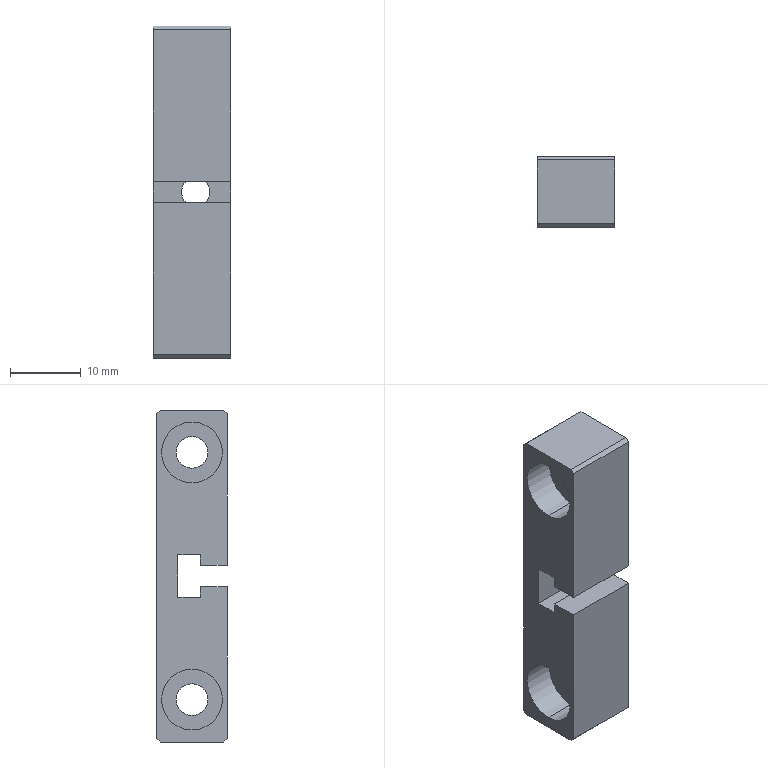Part | NX | features BREP 1 | 1 solid | 30 faces | box 11 x 10 x 47 mm | volume 4061 mm3 | plane 20 | cylinder 10 | commonest cylinder face diameters 4.5 x4 8.6 x4 4 x2
STEP:
#1=CARTESIAN_POINT('',(-1.,0.,-21.8));
#2=VERTEX_POINT('',#1);
#3=CARTESIAN_POINT('',(-1.,0.,-13.2));
#4=VERTEX_POINT('',#3);
#5=CARTESIAN_POINT('',(-1.,0.,-17.5));
#6=DIRECTION('',(-1.,0.,0.));
#7=DIRECTION('',(0.,0.,1.));
#8=AXIS2_PLACEMENT_3D('',#5,#6,#7);
#9=CIRCLE('',#8,4.3);
#10=EDGE_CURVE('',#2,#4,#9,.T.);
#11=ORIENTED_EDGE('',*,*,#10,.F.);
#12=CARTESIAN_POINT('',(-5.5,0.,-21.8));
#13=VERTEX_POINT('',#12);
#14=CARTESIAN_POINT('',(-5.5,0.,-21.8));
#15=DIRECTION('',(-1.,0.,0.));
#16=VECTOR('',#15,1000.);
#17=LINE('',#14,#16);
#18=EDGE_CURVE('',#13,#2,#17,.F.);
#19=ORIENTED_EDGE('',*,*,#18,.F.);
#20=CARTESIAN_POINT('',(-5.5,0.,-13.2));
#21=VERTEX_POINT('',#20);
#22=CARTESIAN_POINT('',(-5.5,0.,-17.5));
#23=DIRECTION('',(-1.,0.,0.));
#24=DIRECTION('',(0.,0.,1.));
#25=AXIS2_PLACEMENT_3D('',#22,#23,#24);
#26=CIRCLE('',#25,4.3);
#27=EDGE_CURVE('',#13,#21,#26,.T.);
#28=ORIENTED_EDGE('',*,*,#27,.T.);
#29=CARTESIAN_POINT('',(-5.5,0.,-13.2));
#30=DIRECTION('',(-1.,0.,0.));
#31=VECTOR('',#30,1000.);
#32=LINE('',#29,#31);
#33=EDGE_CURVE('',#21,#4,#32,.F.);
#34=ORIENTED_EDGE('',*,*,#33,.T.);
#35=EDGE_LOOP('',(#11,#19,#28,#34));
#36=FACE_BOUND('',#35,.T.);
#37=CARTESIAN_POINT('',(-5.5,0.,-17.5));
#38=DIRECTION('',(-1.,0.,0.));
#39=DIRECTION('',(0.,0.,1.));
#40=AXIS2_PLACEMENT_3D('',#37,#38,#39);
#41=CYLINDRICAL_SURFACE('',#40,4.3);
#42=ADVANCED_FACE('',(#36),#41,.F.);
#43=CARTESIAN_POINT('',(5.5,0.,-19.75));
#44=VERTEX_POINT('',#43);
#45=CARTESIAN_POINT('',(5.5,0.,-15.25));
#46=VERTEX_POINT('',#45);
#47=CARTESIAN_POINT('',(5.5,0.,-17.5));
#48=DIRECTION('',(-1.,0.,0.));
#49=DIRECTION('',(0.,0.,1.));
#50=AXIS2_PLACEMENT_3D('',#47,#48,#49);
#51=CIRCLE('',#50,2.25);
#52=EDGE_CURVE('',#44,#46,#51,.T.);
#53=ORIENTED_EDGE('',*,*,#52,.F.);
#54=CARTESIAN_POINT('',(-1.,0.,-19.75));
#55=VERTEX_POINT('',#54);
#56=CARTESIAN_POINT('',(-5.5,0.,-19.75));
#57=DIRECTION('',(-1.,0.,0.));
#58=VECTOR('',#57,1000.);
#59=LINE('',#56,#58);
#60=EDGE_CURVE('',#55,#44,#59,.F.);
#61=ORIENTED_EDGE('',*,*,#60,.F.);
#62=CARTESIAN_POINT('',(-1.,0.,-15.25));
#63=VERTEX_POINT('',#62);
#64=CARTESIAN_POINT('',(-1.,0.,-17.5));
#65=DIRECTION('',(-1.,0.,0.));
#66=DIRECTION('',(0.,0.,1.));
#67=AXIS2_PLACEMENT_3D('',#64,#65,#66);
#68=CIRCLE('',#67,2.25);
#69=EDGE_CURVE('',#55,#63,#68,.T.);
#70=ORIENTED_EDGE('',*,*,#69,.T.);
#71=CARTESIAN_POINT('',(-5.5,0.,-15.25));
#72=DIRECTION('',(-1.,0.,0.));
#73=VECTOR('',#72,1000.);
#74=LINE('',#71,#73);
#75=EDGE_CURVE('',#63,#46,#74,.F.);
#76=ORIENTED_EDGE('',*,*,#75,.T.);
#77=EDGE_LOOP('',(#53,#61,#70,#76));
#78=FACE_BOUND('',#77,.T.);
#79=CARTESIAN_POINT('',(-5.5,0.,-17.5));
#80=DIRECTION('',(-1.,0.,0.));
#81=DIRECTION('',(0.,0.,1.));
#82=AXIS2_PLACEMENT_3D('',#79,#80,#81);
#83=CYLINDRICAL_SURFACE('',#82,2.25);
#84=ADVANCED_FACE('',(#78),#83,.F.);
#85=CARTESIAN_POINT('',(-1.,0.,13.2));
#86=VERTEX_POINT('',#85);
#87=CARTESIAN_POINT('',(-1.,0.,21.8));
#88=VERTEX_POINT('',#87);
#89=CARTESIAN_POINT('',(-1.,0.,17.5));
#90=DIRECTION('',(-1.,0.,0.));
#91=DIRECTION('',(0.,0.,1.));
#92=AXIS2_PLACEMENT_3D('',#89,#90,#91);
#93=CIRCLE('',#92,4.3);
#94=EDGE_CURVE('',#86,#88,#93,.T.);
#95=ORIENTED_EDGE('',*,*,#94,.F.);
#96=CARTESIAN_POINT('',(-5.5,0.,13.2));
#97=VERTEX_POINT('',#96);
#98=CARTESIAN_POINT('',(-5.5,0.,13.2));
#99=DIRECTION('',(-1.,0.,0.));
#100=VECTOR('',#99,1000.);
#101=LINE('',#98,#100);
#102=EDGE_CURVE('',#97,#86,#101,.F.);
#103=ORIENTED_EDGE('',*,*,#102,.F.);
#104=CARTESIAN_POINT('',(-5.5,0.,21.8));
#105=VERTEX_POINT('',#104);
#106=CARTESIAN_POINT('',(-5.5,0.,17.5));
#107=DIRECTION('',(-1.,0.,0.));
#108=DIRECTION('',(0.,0.,1.));
#109=AXIS2_PLACEMENT_3D('',#106,#107,#108);
#110=CIRCLE('',#109,4.3);
#111=EDGE_CURVE('',#97,#105,#110,.T.);
#112=ORIENTED_EDGE('',*,*,#111,.T.);
#113=CARTESIAN_POINT('',(-5.5,0.,21.8));
#114=DIRECTION('',(-1.,0.,0.));
#115=VECTOR('',#114,1000.);
#116=LINE('',#113,#115);
#117=EDGE_CURVE('',#105,#88,#116,.F.);
#118=ORIENTED_EDGE('',*,*,#117,.T.);
#119=EDGE_LOOP('',(#95,#103,#112,#118));
#120=FACE_BOUND('',#119,.T.);
#121=CARTESIAN_POINT('',(-5.5,0.,17.5));
#122=DIRECTION('',(-1.,0.,0.));
#123=DIRECTION('',(0.,0.,1.));
#124=AXIS2_PLACEMENT_3D('',#121,#122,#123);
#125=CYLINDRICAL_SURFACE('',#124,4.3);
#126=ADVANCED_FACE('',(#120),#125,.F.);
#127=CARTESIAN_POINT('',(5.5,0.,15.25));
#128=VERTEX_POINT('',#127);
#129=CARTESIAN_POINT('',(5.5,0.,19.75));
#130=VERTEX_POINT('',#129);
#131=CARTESIAN_POINT('',(5.5,0.,17.5));
#132=DIRECTION('',(-1.,0.,0.));
#133=DIRECTION('',(0.,0.,1.));
#134=AXIS2_PLACEMENT_3D('',#131,#132,#133);
#135=CIRCLE('',#134,2.25);
#136=EDGE_CURVE('',#128,#130,#135,.T.);
#137=ORIENTED_EDGE('',*,*,#136,.F.);
#138=CARTESIAN_POINT('',(-1.,0.,15.25));
#139=VERTEX_POINT('',#138);
#140=CARTESIAN_POINT('',(-5.5,0.,15.25));
#141=DIRECTION('',(-1.,0.,0.));
#142=VECTOR('',#141,1000.);
#143=LINE('',#140,#142);
#144=EDGE_CURVE('',#139,#128,#143,.F.);
#145=ORIENTED_EDGE('',*,*,#144,.F.);
#146=CARTESIAN_POINT('',(-1.,0.,19.75));
#147=VERTEX_POINT('',#146);
#148=CARTESIAN_POINT('',(-1.,0.,17.5));
#149=DIRECTION('',(-1.,0.,0.));
#150=DIRECTION('',(0.,0.,1.));
#151=AXIS2_PLACEMENT_3D('',#148,#149,#150);
#152=CIRCLE('',#151,2.25);
#153=EDGE_CURVE('',#139,#147,#152,.T.);
#154=ORIENTED_EDGE('',*,*,#153,.T.);
#155=CARTESIAN_POINT('',(-5.5,0.,19.75));
#156=DIRECTION('',(-1.,0.,0.));
#157=VECTOR('',#156,1000.);
#158=LINE('',#155,#157);
#159=EDGE_CURVE('',#147,#130,#158,.F.);
#160=ORIENTED_EDGE('',*,*,#159,.T.);
#161=EDGE_LOOP('',(#137,#145,#154,#160));
#162=FACE_BOUND('',#161,.T.);
#163=CARTESIAN_POINT('',(-5.5,0.,17.5));
#164=DIRECTION('',(-1.,0.,0.));
#165=DIRECTION('',(0.,0.,1.));
#166=AXIS2_PLACEMENT_3D('',#163,#164,#165);
#167=CYLINDRICAL_SURFACE('',#166,2.25);
#168=ADVANCED_FACE('',(#162),#167,.F.);
#169=CARTESIAN_POINT('',(0.5,2.,2.));
#170=VERTEX_POINT('',#169);
#171=CARTESIAN_POINT('',(0.5,2.,-2.));
#172=VERTEX_POINT('',#171);
#173=CARTESIAN_POINT('',(0.5,2.,0.));
#174=DIRECTION('',(0.,-1.,0.));
#175=DIRECTION('',(-1.,0.,0.));
#176=AXIS2_PLACEMENT_3D('',#173,#174,#175);
#177=CIRCLE('',#176,2.);
#178=EDGE_CURVE('',#170,#172,#177,.T.);
#179=ORIENTED_EDGE('',*,*,#178,.T.);
#180=CARTESIAN_POINT('',(0.5,5.,-2.));
#181=VERTEX_POINT('',#180);
#182=CARTESIAN_POINT('',(0.5,-5.001,-2.));
#183=DIRECTION('',(0.,1.,0.));
#184=VECTOR('',#183,1000.);
#185=LINE('',#182,#184);
#186=EDGE_CURVE('',#181,#172,#185,.F.);
#187=ORIENTED_EDGE('',*,*,#186,.F.);
#188=CARTESIAN_POINT('',(0.5,5.,2.));
#189=VERTEX_POINT('',#188);
#190=CARTESIAN_POINT('',(0.5,5.,0.));
#191=DIRECTION('',(0.,1.,0.));
#192=DIRECTION('',(0.,0.,1.));
#193=AXIS2_PLACEMENT_3D('',#190,#191,#192);
#194=CIRCLE('',#193,2.);
#195=EDGE_CURVE('',#181,#189,#194,.T.);
#196=ORIENTED_EDGE('',*,*,#195,.T.);
#197=CARTESIAN_POINT('',(0.5,-5.001,2.));
#198=DIRECTION('',(0.,1.,0.));
#199=VECTOR('',#198,1000.);
#200=LINE('',#197,#199);
#201=EDGE_CURVE('',#189,#170,#200,.F.);
#202=ORIENTED_EDGE('',*,*,#201,.T.);
#203=EDGE_LOOP('',(#179,#187,#196,#202));
#204=FACE_BOUND('',#203,.T.);
#205=CARTESIAN_POINT('',(0.5,-5.001,0.));
#206=DIRECTION('',(0.,1.,0.));
#207=DIRECTION('',(0.,0.,1.));
#208=AXIS2_PLACEMENT_3D('',#205,#206,#207);
#209=CYLINDRICAL_SURFACE('',#208,2.);
#210=ADVANCED_FACE('',(#204),#209,.F.);
#211=CARTESIAN_POINT('',(-5.5,-5.,-23.));
#212=VERTEX_POINT('',#211);
#213=CARTESIAN_POINT('',(-5.5,-5.,-1.5));
#214=VERTEX_POINT('',#213);
#215=CARTESIAN_POINT('',(-5.5,-5.,-23.5));
#216=DIRECTION('',(0.,0.,1.));
#217=VECTOR('',#216,1000.);
#218=LINE('',#215,#217);
#219=EDGE_CURVE('',#212,#214,#218,.T.);
#220=ORIENTED_EDGE('',*,*,#219,.F.);
#221=CARTESIAN_POINT('',(5.5,-5.,-23.));
#222=VERTEX_POINT('',#221);
#223=CARTESIAN_POINT('',(-5.5,-5.,-23.));
#224=DIRECTION('',(1.,0.,0.));
#225=VECTOR('',#224,1000.);
#226=LINE('',#223,#225);
#227=EDGE_CURVE('',#212,#222,#226,.T.);
#228=ORIENTED_EDGE('',*,*,#227,.T.);
#229=CARTESIAN_POINT('',(5.5,-5.,-1.5));
#230=VERTEX_POINT('',#229);
#231=CARTESIAN_POINT('',(5.5,-5.,-23.5));
#232=DIRECTION('',(0.,0.,1.));
#233=VECTOR('',#232,1000.);
#234=LINE('',#231,#233);
#235=EDGE_CURVE('',#222,#230,#234,.T.);
#236=ORIENTED_EDGE('',*,*,#235,.T.);
#237=CARTESIAN_POINT('',(5.5,-5.,-1.5));
#238=DIRECTION('',(-1.,0.,0.));
#239=VECTOR('',#238,1000.);
#240=LINE('',#237,#239);
#241=EDGE_CURVE('',#230,#214,#240,.T.);
#242=ORIENTED_EDGE('',*,*,#241,.T.);
#243=EDGE_LOOP('',(#220,#228,#236,#242));
#244=FACE_BOUND('',#243,.T.);
#245=CARTESIAN_POINT('',(-5.5,-5.,-23.5));
#246=DIRECTION('',(0.,-1.,0.));
#247=DIRECTION('',(0.,0.,-1.));
#248=AXIS2_PLACEMENT_3D('',#245,#246,#247);
#249=PLANE('',#248);
#250=ADVANCED_FACE('',(#244),#249,.T.);
#251=CARTESIAN_POINT('',(-5.5,-1.2,-3.));
#252=VERTEX_POINT('',#251);
#253=CARTESIAN_POINT('',(-5.5,-1.2,-1.5));
#254=VERTEX_POINT('',#253);
#255=CARTESIAN_POINT('',(-5.5,-1.2,-3.));
#256=DIRECTION('',(0.,0.,1.));
#257=VECTOR('',#256,1000.);
#258=LINE('',#255,#257);
#259=EDGE_CURVE('',#252,#254,#258,.T.);
#260=ORIENTED_EDGE('',*,*,#259,.T.);
#261=CARTESIAN_POINT('',(5.5,-1.2,-1.5));
#262=VERTEX_POINT('',#261);
#263=CARTESIAN_POINT('',(5.5,-1.2,-1.5));
#264=DIRECTION('',(-1.,0.,0.));
#265=VECTOR('',#264,1000.);
#266=LINE('',#263,#265);
#267=EDGE_CURVE('',#262,#254,#266,.T.);
#268=ORIENTED_EDGE('',*,*,#267,.F.);
#269=CARTESIAN_POINT('',(5.5,-1.2,-3.));
#270=VERTEX_POINT('',#269);
#271=CARTESIAN_POINT('',(5.5,-1.2,-3.));
#272=DIRECTION('',(0.,0.,1.));
#273=VECTOR('',#272,1000.);
#274=LINE('',#271,#273);
#275=EDGE_CURVE('',#270,#262,#274,.T.);
#276=ORIENTED_EDGE('',*,*,#275,.F.);
#277=CARTESIAN_POINT('',(5.5,-1.2,-3.));
#278=DIRECTION('',(-1.,0.,0.));
#279=VECTOR('',#278,1000.);
#280=LINE('',#277,#279);
#281=EDGE_CURVE('',#270,#252,#280,.T.);
#282=ORIENTED_EDGE('',*,*,#281,.T.);
#283=EDGE_LOOP('',(#260,#268,#276,#282));
#284=FACE_BOUND('',#283,.T.);
#285=CARTESIAN_POINT('',(5.5,-1.2,-3.));
#286=DIRECTION('',(0.,-1.,0.));
#287=DIRECTION('',(0.,0.,-1.));
#288=AXIS2_PLACEMENT_3D('',#285,#286,#287);
#289=PLANE('',#288);
#290=ADVANCED_FACE('',(#284),#289,.F.);
#291=CARTESIAN_POINT('',(-5.5,-5.,1.5));
#292=VERTEX_POINT('',#291);
#293=CARTESIAN_POINT('',(-5.5,-5.,23.));
#294=VERTEX_POINT('',#293);
#295=CARTESIAN_POINT('',(-5.5,-5.,-23.5));
#296=DIRECTION('',(0.,0.,1.));
#297=VECTOR('',#296,1000.);
#298=LINE('',#295,#297);
#299=EDGE_CURVE('',#292,#294,#298,.T.);
#300=ORIENTED_EDGE('',*,*,#299,.T.);
#301=CARTESIAN_POINT('',(-5.5,-4.5,23.5));
#302=VERTEX_POINT('',#301);
#303=CARTESIAN_POINT('',(-5.5,-28.25,-0.25));
#304=DIRECTION('',(0.,0.7071,0.7071));
#305=VECTOR('',#304,1000.);
#306=LINE('',#303,#305);
#307=EDGE_CURVE('',#294,#302,#306,.T.);
#308=ORIENTED_EDGE('',*,*,#307,.T.);
#309=CARTESIAN_POINT('',(-5.5,4.5,23.5));
#310=VERTEX_POINT('',#309);
#311=CARTESIAN_POINT('',(-5.5,-5.,23.5));
#312=DIRECTION('',(0.,-1.,0.));
#313=VECTOR('',#312,1000.);
#314=LINE('',#311,#313);
#315=EDGE_CURVE('',#310,#302,#314,.T.);
#316=ORIENTED_EDGE('',*,*,#315,.F.);
#317=CARTESIAN_POINT('',(-5.5,5.,23.));
#318=VERTEX_POINT('',#317);
#319=CARTESIAN_POINT('',(-5.5,23.25,4.75));
#320=DIRECTION('',(0.,0.7071,-0.7071));
#321=VECTOR('',#320,1000.);
#322=LINE('',#319,#321);
#323=EDGE_CURVE('',#310,#318,#322,.T.);
#324=ORIENTED_EDGE('',*,*,#323,.T.);
#325=CARTESIAN_POINT('',(-5.5,5.,-23.));
#326=VERTEX_POINT('',#325);
#327=CARTESIAN_POINT('',(-5.5,5.,-23.5));
#328=DIRECTION('',(0.,0.,1.));
#329=VECTOR('',#328,1000.);
#330=LINE('',#327,#329);
#331=EDGE_CURVE('',#326,#318,#330,.T.);
#332=ORIENTED_EDGE('',*,*,#331,.F.);
#333=CARTESIAN_POINT('',(-5.5,4.5,-23.5));
#334=VERTEX_POINT('',#333);
#335=CARTESIAN_POINT('',(-5.5,-0.25,-28.25));
#336=DIRECTION('',(0.,-0.7071,-0.7071));
#337=VECTOR('',#336,1000.);
#338=LINE('',#335,#337);
#339=EDGE_CURVE('',#326,#334,#338,.T.);
#340=ORIENTED_EDGE('',*,*,#339,.T.);
#341=CARTESIAN_POINT('',(-5.5,-4.5,-23.5));
#342=VERTEX_POINT('',#341);
#343=CARTESIAN_POINT('',(-5.5,-5.,-23.5));
#344=DIRECTION('',(0.,-1.,0.));
#345=VECTOR('',#344,1000.);
#346=LINE('',#343,#345);
#347=EDGE_CURVE('',#334,#342,#346,.T.);
#348=ORIENTED_EDGE('',*,*,#347,.T.);
#349=CARTESIAN_POINT('',(-5.5,-4.75,-23.25));
#350=DIRECTION('',(0.,-0.7071,0.7071));
#351=VECTOR('',#350,1000.);
#352=LINE('',#349,#351);
#353=EDGE_CURVE('',#342,#212,#352,.T.);
#354=ORIENTED_EDGE('',*,*,#353,.T.);
#355=ORIENTED_EDGE('',*,*,#219,.T.);
#356=CARTESIAN_POINT('',(-5.5,-1.2,-1.5));
#357=DIRECTION('',(0.,-1.,0.));
#358=VECTOR('',#357,1000.);
#359=LINE('',#356,#358);
#360=EDGE_CURVE('',#254,#214,#359,.T.);
#361=ORIENTED_EDGE('',*,*,#360,.F.);
#362=ORIENTED_EDGE('',*,*,#259,.F.);
#363=CARTESIAN_POINT('',(-5.5,2.,-3.));
#364=VERTEX_POINT('',#363);
#365=CARTESIAN_POINT('',(-5.5,2.,-3.));
#366=DIRECTION('',(0.,-1.,0.));
#367=VECTOR('',#366,1000.);
#368=LINE('',#365,#367);
#369=EDGE_CURVE('',#364,#252,#368,.T.);
#370=ORIENTED_EDGE('',*,*,#369,.F.);
#371=CARTESIAN_POINT('',(-5.5,2.,3.));
#372=VERTEX_POINT('',#371);
#373=CARTESIAN_POINT('',(-5.5,2.,-3.));
#374=DIRECTION('',(0.,0.,-1.));
#375=VECTOR('',#374,1000.);
#376=LINE('',#373,#375);
#377=EDGE_CURVE('',#372,#364,#376,.T.);
#378=ORIENTED_EDGE('',*,*,#377,.F.);
#379=CARTESIAN_POINT('',(-5.5,-1.2,3.));
#380=VERTEX_POINT('',#379);
#381=CARTESIAN_POINT('',(-5.5,2.,3.));
#382=DIRECTION('',(0.,1.,0.));
#383=VECTOR('',#382,1000.);
#384=LINE('',#381,#383);
#385=EDGE_CURVE('',#380,#372,#384,.T.);
#386=ORIENTED_EDGE('',*,*,#385,.F.);
#387=CARTESIAN_POINT('',(-5.5,-1.2,1.5));
#388=VERTEX_POINT('',#387);
#389=CARTESIAN_POINT('',(-5.5,-1.2,-3.));
#390=DIRECTION('',(0.,0.,1.));
#391=VECTOR('',#390,1000.);
#392=LINE('',#389,#391);
#393=EDGE_CURVE('',#388,#380,#392,.T.);
#394=ORIENTED_EDGE('',*,*,#393,.F.);
#395=CARTESIAN_POINT('',(-5.5,-1.2,1.5));
#396=DIRECTION('',(0.,1.,0.));
#397=VECTOR('',#396,1000.);
#398=LINE('',#395,#397);
#399=EDGE_CURVE('',#292,#388,#398,.T.);
#400=ORIENTED_EDGE('',*,*,#399,.F.);
#401=EDGE_LOOP('',(#300,#308,#316,#324,#332,#340,#348,#354,#355,#361,#362,#370,#378,#386,#394,#400));
#402=FACE_BOUND('',#401,.T.);
#403=CARTESIAN_POINT('',(-5.5,0.,-17.5));
#404=DIRECTION('',(-1.,0.,0.));
#405=DIRECTION('',(0.,0.,1.));
#406=AXIS2_PLACEMENT_3D('',#403,#404,#405);
#407=CIRCLE('',#406,4.3);
#408=EDGE_CURVE('',#21,#13,#407,.T.);
#409=ORIENTED_EDGE('',*,*,#408,.F.);
#410=ORIENTED_EDGE('',*,*,#27,.F.);
#411=EDGE_LOOP('',(#409,#410));
#412=FACE_BOUND('',#411,.T.);
#413=CARTESIAN_POINT('',(-5.5,0.,17.5));
#414=DIRECTION('',(-1.,0.,0.));
#415=DIRECTION('',(0.,0.,1.));
#416=AXIS2_PLACEMENT_3D('',#413,#414,#415);
#417=CIRCLE('',#416,4.3);
#418=EDGE_CURVE('',#105,#97,#417,.T.);
#419=ORIENTED_EDGE('',*,*,#418,.F.);
#420=ORIENTED_EDGE('',*,*,#111,.F.);
#421=EDGE_LOOP('',(#419,#420));
#422=FACE_BOUND('',#421,.T.);
#423=CARTESIAN_POINT('',(-5.5,-5.,-23.5));
#424=DIRECTION('',(-1.,0.,0.));
#425=DIRECTION('',(0.,0.,1.));
#426=AXIS2_PLACEMENT_3D('',#423,#424,#425);
#427=PLANE('',#426);
#428=ADVANCED_FACE('',(#402,#412,#422),#427,.T.);
#429=ORIENTED_EDGE('',*,*,#331,.T.);
#430=CARTESIAN_POINT('',(5.5,5.,23.));
#431=VERTEX_POINT('',#430);
#432=CARTESIAN_POINT('',(5.5,5.,23.));
#433=DIRECTION('',(1.,0.,0.));
#434=VECTOR('',#433,1000.);
#435=LINE('',#432,#434);
#436=EDGE_CURVE('',#318,#431,#435,.T.);
#437=ORIENTED_EDGE('',*,*,#436,.T.);
#438=CARTESIAN_POINT('',(5.5,5.,-23.));
#439=VERTEX_POINT('',#438);
#440=CARTESIAN_POINT('',(5.5,5.,-23.5));
#441=DIRECTION('',(0.,0.,1.));
#442=VECTOR('',#441,1000.);
#443=LINE('',#440,#442);
#444=EDGE_CURVE('',#439,#431,#443,.T.);
#445=ORIENTED_EDGE('',*,*,#444,.F.);
#446=CARTESIAN_POINT('',(-5.5,5.,-23.));
#447=DIRECTION('',(-1.,0.,0.));
#448=VECTOR('',#447,1000.);
#449=LINE('',#446,#448);
#450=EDGE_CURVE('',#439,#326,#449,.T.);
#451=ORIENTED_EDGE('',*,*,#450,.T.);
#452=EDGE_LOOP('',(#429,#437,#445,#451));
#453=FACE_BOUND('',#452,.T.);
#454=CARTESIAN_POINT('',(0.5,5.,0.));
#455=DIRECTION('',(0.,1.,0.));
#456=DIRECTION('',(0.,0.,1.));
#457=AXIS2_PLACEMENT_3D('',#454,#455,#456);
#458=CIRCLE('',#457,2.);
#459=EDGE_CURVE('',#189,#181,#458,.T.);
#460=ORIENTED_EDGE('',*,*,#459,.F.);
#461=ORIENTED_EDGE('',*,*,#195,.F.);
#462=EDGE_LOOP('',(#460,#461));
#463=FACE_BOUND('',#462,.T.);
#464=CARTESIAN_POINT('',(-5.5,5.,-23.5));
#465=DIRECTION('',(0.,1.,0.));
#466=DIRECTION('',(1.,0.,0.));
#467=AXIS2_PLACEMENT_3D('',#464,#465,#466);
#468=PLANE('',#467);
#469=ADVANCED_FACE('',(#453,#463),#468,.T.);
#470=CARTESIAN_POINT('',(5.5,-4.5,23.5));
#471=VERTEX_POINT('',#470);
#472=CARTESIAN_POINT('',(5.5,4.5,23.5));
#473=VERTEX_POINT('',#472);
#474=CARTESIAN_POINT('',(5.5,-5.,23.5));
#475=DIRECTION('',(0.,1.,0.));
#476=VECTOR('',#475,1000.);
#477=LINE('',#474,#476);
#478=EDGE_CURVE('',#471,#473,#477,.T.);
#479=ORIENTED_EDGE('',*,*,#478,.F.);
#480=CARTESIAN_POINT('',(5.5,-5.,23.));
#481=VERTEX_POINT('',#480);
#482=CARTESIAN_POINT('',(5.5,-28.25,-0.25));
#483=DIRECTION('',(0.,-0.7071,-0.7071));
#484=VECTOR('',#483,1000.);
#485=LINE('',#482,#484);
#486=EDGE_CURVE('',#471,#481,#485,.T.);
#487=ORIENTED_EDGE('',*,*,#486,.T.);
#488=CARTESIAN_POINT('',(5.5,-5.,1.5));
#489=VERTEX_POINT('',#488);
#490=CARTESIAN_POINT('',(5.5,-5.,-23.5));
#491=DIRECTION('',(0.,0.,1.));
#492=VECTOR('',#491,1000.);
#493=LINE('',#490,#492);
#494=EDGE_CURVE('',#489,#481,#493,.T.);
#495=ORIENTED_EDGE('',*,*,#494,.F.);
#496=CARTESIAN_POINT('',(5.5,-1.2,1.5));
#497=VERTEX_POINT('',#496);
#498=CARTESIAN_POINT('',(5.5,-1.2,1.5));
#499=DIRECTION('',(0.,1.,0.));
#500=VECTOR('',#499,1000.);
#501=LINE('',#498,#500);
#502=EDGE_CURVE('',#489,#497,#501,.T.);
#503=ORIENTED_EDGE('',*,*,#502,.T.);
#504=CARTESIAN_POINT('',(5.5,-1.2,3.));
#505=VERTEX_POINT('',#504);
#506=CARTESIAN_POINT('',(5.5,-1.2,-3.));
#507=DIRECTION('',(0.,0.,1.));
#508=VECTOR('',#507,1000.);
#509=LINE('',#506,#508);
#510=EDGE_CURVE('',#497,#505,#509,.T.);
#511=ORIENTED_EDGE('',*,*,#510,.T.);
#512=CARTESIAN_POINT('',(5.5,2.,3.));
#513=VERTEX_POINT('',#512);
#514=CARTESIAN_POINT('',(5.5,2.,3.));
#515=DIRECTION('',(0.,1.,0.));
#516=VECTOR('',#515,1000.);
#517=LINE('',#514,#516);
#518=EDGE_CURVE('',#505,#513,#517,.T.);
#519=ORIENTED_EDGE('',*,*,#518,.T.);
#520=CARTESIAN_POINT('',(5.5,2.,-3.));
#521=VERTEX_POINT('',#520);
#522=CARTESIAN_POINT('',(5.5,2.,-3.));
#523=DIRECTION('',(0.,0.,-1.));
#524=VECTOR('',#523,1000.);
#525=LINE('',#522,#524);
#526=EDGE_CURVE('',#513,#521,#525,.T.);
#527=ORIENTED_EDGE('',*,*,#526,.T.);
#528=CARTESIAN_POINT('',(5.5,2.,-3.));
#529=DIRECTION('',(0.,-1.,0.));
#530=VECTOR('',#529,1000.);
#531=LINE('',#528,#530);
#532=EDGE_CURVE('',#521,#270,#531,.T.);
#533=ORIENTED_EDGE('',*,*,#532,.T.);
#534=ORIENTED_EDGE('',*,*,#275,.T.);
#535=CARTESIAN_POINT('',(5.5,-1.2,-1.5));
#536=DIRECTION('',(0.,-1.,0.));
#537=VECTOR('',#536,1000.);
#538=LINE('',#535,#537);
#539=EDGE_CURVE('',#262,#230,#538,.T.);
#540=ORIENTED_EDGE('',*,*,#539,.T.);
#541=ORIENTED_EDGE('',*,*,#235,.F.);
#542=CARTESIAN_POINT('',(5.5,-4.5,-23.5));
#543=VERTEX_POINT('',#542);
#544=CARTESIAN_POINT('',(5.5,-4.75,-23.25));
#545=DIRECTION('',(0.,0.7071,-0.7071));
#546=VECTOR('',#545,1000.);
#547=LINE('',#544,#546);
#548=EDGE_CURVE('',#222,#543,#547,.T.);
#549=ORIENTED_EDGE('',*,*,#548,.T.);
#550=CARTESIAN_POINT('',(5.5,4.5,-23.5));
#551=VERTEX_POINT('',#550);
#552=CARTESIAN_POINT('',(5.5,-5.,-23.5));
#553=DIRECTION('',(0.,1.,0.));
#554=VECTOR('',#553,1000.);
#555=LINE('',#552,#554);
#556=EDGE_CURVE('',#543,#551,#555,.T.);
#557=ORIENTED_EDGE('',*,*,#556,.T.);
#558=CARTESIAN_POINT('',(5.5,-0.25,-28.25));
#559=DIRECTION('',(0.,0.7071,0.7071));
#560=VECTOR('',#559,1000.);
#561=LINE('',#558,#560);
#562=EDGE_CURVE('',#551,#439,#561,.T.);
#563=ORIENTED_EDGE('',*,*,#562,.T.);
#564=ORIENTED_EDGE('',*,*,#444,.T.);
#565=CARTESIAN_POINT('',(5.5,23.25,4.75));
#566=DIRECTION('',(0.,-0.7071,0.7071));
#567=VECTOR('',#566,1000.);
#568=LINE('',#565,#567);
#569=EDGE_CURVE('',#431,#473,#568,.T.);
#570=ORIENTED_EDGE('',*,*,#569,.T.);
#571=EDGE_LOOP('',(#479,#487,#495,#503,#511,#519,#527,#533,#534,#540,#541,#549,#557,#563,#564,#570));
#572=FACE_BOUND('',#571,.T.);
#573=CARTESIAN_POINT('',(5.5,0.,-17.5));
#574=DIRECTION('',(-1.,0.,0.));
#575=DIRECTION('',(0.,0.,1.));
#576=AXIS2_PLACEMENT_3D('',#573,#574,#575);
#577=CIRCLE('',#576,2.25);
#578=EDGE_CURVE('',#46,#44,#577,.T.);
#579=ORIENTED_EDGE('',*,*,#578,.T.);
#580=ORIENTED_EDGE('',*,*,#52,.T.);
#581=EDGE_LOOP('',(#579,#580));
#582=FACE_BOUND('',#581,.T.);
#583=CARTESIAN_POINT('',(5.5,0.,17.5));
#584=DIRECTION('',(-1.,0.,0.));
#585=DIRECTION('',(0.,0.,1.));
#586=AXIS2_PLACEMENT_3D('',#583,#584,#585);
#587=CIRCLE('',#586,2.25);
#588=EDGE_CURVE('',#130,#128,#587,.T.);
#589=ORIENTED_EDGE('',*,*,#588,.T.);
#590=ORIENTED_EDGE('',*,*,#136,.T.);
#591=EDGE_LOOP('',(#589,#590));
#592=FACE_BOUND('',#591,.T.);
#593=CARTESIAN_POINT('',(5.5,-5.,-23.5));
#594=DIRECTION('',(1.,0.,0.));
#595=DIRECTION('',(0.,1.,0.));
#596=AXIS2_PLACEMENT_3D('',#593,#594,#595);
#597=PLANE('',#596);
#598=ADVANCED_FACE('',(#572,#582,#592),#597,.T.);
#599=ORIENTED_EDGE('',*,*,#494,.T.);
#600=CARTESIAN_POINT('',(-5.5,-5.,23.));
#601=DIRECTION('',(-1.,0.,0.));
#602=VECTOR('',#601,1000.);
#603=LINE('',#600,#602);
#604=EDGE_CURVE('',#481,#294,#603,.T.);
#605=ORIENTED_EDGE('',*,*,#604,.T.);
#606=ORIENTED_EDGE('',*,*,#299,.F.);
#607=CARTESIAN_POINT('',(5.5,-5.,1.5));
#608=DIRECTION('',(-1.,0.,0.));
#609=VECTOR('',#608,1000.);
#610=LINE('',#607,#609);
#611=EDGE_CURVE('',#489,#292,#610,.T.);
#612=ORIENTED_EDGE('',*,*,#611,.F.);
#613=EDGE_LOOP('',(#599,#605,#606,#612));
#614=FACE_BOUND('',#613,.T.);
#615=CARTESIAN_POINT('',(-5.5,-5.,-23.5));
#616=DIRECTION('',(0.,-1.,0.));
#617=DIRECTION('',(0.,0.,-1.));
#618=AXIS2_PLACEMENT_3D('',#615,#616,#617);
#619=PLANE('',#618);
#620=ADVANCED_FACE('',(#614),#619,.T.);
#621=ORIENTED_EDGE('',*,*,#556,.F.);
#622=CARTESIAN_POINT('',(-5.5,-4.5,-23.5));
#623=DIRECTION('',(-1.,0.,0.));
#624=VECTOR('',#623,1000.);
#625=LINE('',#622,#624);
#626=EDGE_CURVE('',#543,#342,#625,.T.);
#627=ORIENTED_EDGE('',*,*,#626,.T.);
#628=ORIENTED_EDGE('',*,*,#347,.F.);
#629=CARTESIAN_POINT('',(-5.5,4.5,-23.5));
#630=DIRECTION('',(1.,0.,0.));
#631=VECTOR('',#630,1000.);
#632=LINE('',#629,#631);
#633=EDGE_CURVE('',#334,#551,#632,.T.);
#634=ORIENTED_EDGE('',*,*,#633,.T.);
#635=EDGE_LOOP('',(#621,#627,#628,#634));
#636=FACE_BOUND('',#635,.T.);
#637=CARTESIAN_POINT('',(-5.5,5.,-23.5));
#638=DIRECTION('',(0.,0.,-1.));
#639=DIRECTION('',(0.,-1.,0.));
#640=AXIS2_PLACEMENT_3D('',#637,#638,#639);
#641=PLANE('',#640);
#642=ADVANCED_FACE('',(#636),#641,.T.);
#643=ORIENTED_EDGE('',*,*,#315,.T.);
#644=CARTESIAN_POINT('',(5.5,-4.5,23.5));
#645=DIRECTION('',(1.,0.,0.));
#646=VECTOR('',#645,1000.);
#647=LINE('',#644,#646);
#648=EDGE_CURVE('',#302,#471,#647,.T.);
#649=ORIENTED_EDGE('',*,*,#648,.T.);
#650=ORIENTED_EDGE('',*,*,#478,.T.);
#651=CARTESIAN_POINT('',(-5.5,4.5,23.5));
#652=DIRECTION('',(-1.,0.,0.));
#653=VECTOR('',#652,1000.);
#654=LINE('',#651,#653);
#655=EDGE_CURVE('',#473,#310,#654,.T.);
#656=ORIENTED_EDGE('',*,*,#655,.T.);
#657=EDGE_LOOP('',(#643,#649,#650,#656));
#658=FACE_BOUND('',#657,.T.);
#659=CARTESIAN_POINT('',(-5.5,5.,23.5));
#660=DIRECTION('',(0.,0.,-1.));
#661=DIRECTION('',(0.,-1.,0.));
#662=AXIS2_PLACEMENT_3D('',#659,#660,#661);
#663=PLANE('',#662);
#664=ADVANCED_FACE('',(#658),#663,.F.);
#665=ORIENTED_EDGE('',*,*,#369,.T.);
#666=ORIENTED_EDGE('',*,*,#281,.F.);
#667=ORIENTED_EDGE('',*,*,#532,.F.);
#668=CARTESIAN_POINT('',(5.5,2.,-3.));
#669=DIRECTION('',(-1.,0.,0.));
#670=VECTOR('',#669,1000.);
#671=LINE('',#668,#670);
#672=EDGE_CURVE('',#521,#364,#671,.T.);
#673=ORIENTED_EDGE('',*,*,#672,.T.);
#674=EDGE_LOOP('',(#665,#666,#667,#673));
#675=FACE_BOUND('',#674,.T.);
#676=CARTESIAN_POINT('',(5.5,2.,-3.));
#677=DIRECTION('',(0.,0.,-1.));
#678=DIRECTION('',(-1.,0.,0.));
#679=AXIS2_PLACEMENT_3D('',#676,#677,#678);
#680=PLANE('',#679);
#681=ADVANCED_FACE('',(#675),#680,.F.);
#682=ORIENTED_EDGE('',*,*,#377,.T.);
#683=ORIENTED_EDGE('',*,*,#672,.F.);
#684=ORIENTED_EDGE('',*,*,#526,.F.);
#685=CARTESIAN_POINT('',(5.5,2.,3.));
#686=DIRECTION('',(-1.,0.,0.));
#687=VECTOR('',#686,1000.);
#688=LINE('',#685,#687);
#689=EDGE_CURVE('',#513,#372,#688,.T.);
#690=ORIENTED_EDGE('',*,*,#689,.T.);
#691=EDGE_LOOP('',(#682,#683,#684,#690));
#692=FACE_BOUND('',#691,.T.);
#693=ORIENTED_EDGE('',*,*,#178,.F.);
#694=CARTESIAN_POINT('',(0.5,2.,0.));
#695=DIRECTION('',(0.,-1.,0.));
#696=DIRECTION('',(-1.,0.,0.));
#697=AXIS2_PLACEMENT_3D('',#694,#695,#696);
#698=CIRCLE('',#697,2.);
#699=EDGE_CURVE('',#172,#170,#698,.T.);
#700=ORIENTED_EDGE('',*,*,#699,.F.);
#701=EDGE_LOOP('',(#693,#700));
#702=FACE_BOUND('',#701,.T.);
#703=CARTESIAN_POINT('',(5.5,2.,-3.));
#704=DIRECTION('',(0.,1.,0.));
#705=DIRECTION('',(1.,0.,0.));
#706=AXIS2_PLACEMENT_3D('',#703,#704,#705);
#707=PLANE('',#706);
#708=ADVANCED_FACE('',(#692,#702),#707,.F.);
#709=ORIENTED_EDGE('',*,*,#385,.T.);
#710=ORIENTED_EDGE('',*,*,#689,.F.);
#711=ORIENTED_EDGE('',*,*,#518,.F.);
#712=CARTESIAN_POINT('',(5.5,-1.2,3.));
#713=DIRECTION('',(-1.,0.,0.));
#714=VECTOR('',#713,1000.);
#715=LINE('',#712,#714);
#716=EDGE_CURVE('',#505,#380,#715,.T.);
#717=ORIENTED_EDGE('',*,*,#716,.T.);
#718=EDGE_LOOP('',(#709,#710,#711,#717));
#719=FACE_BOUND('',#718,.T.);
#720=CARTESIAN_POINT('',(5.5,2.,3.));
#721=DIRECTION('',(0.,0.,1.));
#722=DIRECTION('',(0.,-1.,0.));
#723=AXIS2_PLACEMENT_3D('',#720,#721,#722);
#724=PLANE('',#723);
#725=ADVANCED_FACE('',(#719),#724,.F.);
#726=ORIENTED_EDGE('',*,*,#510,.F.);
#727=CARTESIAN_POINT('',(5.5,-1.2,1.5));
#728=DIRECTION('',(-1.,0.,0.));
#729=VECTOR('',#728,1000.);
#730=LINE('',#727,#729);
#731=EDGE_CURVE('',#497,#388,#730,.T.);
#732=ORIENTED_EDGE('',*,*,#731,.T.);
#733=ORIENTED_EDGE('',*,*,#393,.T.);
#734=ORIENTED_EDGE('',*,*,#716,.F.);
#735=EDGE_LOOP('',(#726,#732,#733,#734));
#736=FACE_BOUND('',#735,.T.);
#737=CARTESIAN_POINT('',(5.5,-1.2,-3.));
#738=DIRECTION('',(0.,-1.,0.));
#739=DIRECTION('',(0.,0.,-1.));
#740=AXIS2_PLACEMENT_3D('',#737,#738,#739);
#741=PLANE('',#740);
#742=ADVANCED_FACE('',(#736),#741,.F.);
#743=ORIENTED_EDGE('',*,*,#399,.T.);
#744=ORIENTED_EDGE('',*,*,#731,.F.);
#745=ORIENTED_EDGE('',*,*,#502,.F.);
#746=ORIENTED_EDGE('',*,*,#611,.T.);
#747=EDGE_LOOP('',(#743,#744,#745,#746));
#748=FACE_BOUND('',#747,.T.);
#749=CARTESIAN_POINT('',(5.5,-1.2,1.5));
#750=DIRECTION('',(0.,0.,1.));
#751=DIRECTION('',(0.,-1.,0.));
#752=AXIS2_PLACEMENT_3D('',#749,#750,#751);
#753=PLANE('',#752);
#754=ADVANCED_FACE('',(#748),#753,.F.);
#755=ORIENTED_EDGE('',*,*,#360,.T.);
#756=ORIENTED_EDGE('',*,*,#241,.F.);
#757=ORIENTED_EDGE('',*,*,#539,.F.);
#758=ORIENTED_EDGE('',*,*,#267,.T.);
#759=EDGE_LOOP('',(#755,#756,#757,#758));
#760=FACE_BOUND('',#759,.T.);
#761=CARTESIAN_POINT('',(5.5,-1.2,-1.5));
#762=DIRECTION('',(0.,0.,-1.));
#763=DIRECTION('',(0.,-1.,0.));
#764=AXIS2_PLACEMENT_3D('',#761,#762,#763);
#765=PLANE('',#764);
#766=ADVANCED_FACE('',(#760),#765,.F.);
#767=ORIENTED_EDGE('',*,*,#186,.T.);
#768=ORIENTED_EDGE('',*,*,#699,.T.);
#769=ORIENTED_EDGE('',*,*,#201,.F.);
#770=ORIENTED_EDGE('',*,*,#459,.T.);
#771=EDGE_LOOP('',(#767,#768,#769,#770));
#772=FACE_BOUND('',#771,.T.);
#773=CARTESIAN_POINT('',(0.5,-5.001,0.));
#774=DIRECTION('',(0.,1.,0.));
#775=DIRECTION('',(0.,0.,1.));
#776=AXIS2_PLACEMENT_3D('',#773,#774,#775);
#777=CYLINDRICAL_SURFACE('',#776,2.);
#778=ADVANCED_FACE('',(#772),#777,.F.);
#779=ORIENTED_EDGE('',*,*,#307,.F.);
#780=ORIENTED_EDGE('',*,*,#604,.F.);
#781=ORIENTED_EDGE('',*,*,#486,.F.);
#782=ORIENTED_EDGE('',*,*,#648,.F.);
#783=EDGE_LOOP('',(#779,#780,#781,#782));
#784=FACE_BOUND('',#783,.T.);
#785=CARTESIAN_POINT('',(-5.5,-4.5,23.5));
#786=DIRECTION('',(0.,-0.7071,0.7071));
#787=DIRECTION('',(-1.,0.,0.));
#788=AXIS2_PLACEMENT_3D('',#785,#786,#787);
#789=PLANE('',#788);
#790=ADVANCED_FACE('',(#784),#789,.T.);
#791=ORIENTED_EDGE('',*,*,#569,.F.);
#792=ORIENTED_EDGE('',*,*,#436,.F.);
#793=ORIENTED_EDGE('',*,*,#323,.F.);
#794=ORIENTED_EDGE('',*,*,#655,.F.);
#795=EDGE_LOOP('',(#791,#792,#793,#794));
#796=FACE_BOUND('',#795,.T.);
#797=CARTESIAN_POINT('',(-5.5,4.5,23.5));
#798=DIRECTION('',(0.,0.7071,0.7071));
#799=DIRECTION('',(1.,0.,0.));
#800=AXIS2_PLACEMENT_3D('',#797,#798,#799);
#801=PLANE('',#800);
#802=ADVANCED_FACE('',(#796),#801,.T.);
#803=ORIENTED_EDGE('',*,*,#353,.F.);
#804=ORIENTED_EDGE('',*,*,#626,.F.);
#805=ORIENTED_EDGE('',*,*,#548,.F.);
#806=ORIENTED_EDGE('',*,*,#227,.F.);
#807=EDGE_LOOP('',(#803,#804,#805,#806));
#808=FACE_BOUND('',#807,.T.);
#809=CARTESIAN_POINT('',(-5.5,-5.,-23.));
#810=DIRECTION('',(0.,0.7071,0.7071));
#811=DIRECTION('',(1.,0.,0.));
#812=AXIS2_PLACEMENT_3D('',#809,#810,#811);
#813=PLANE('',#812);
#814=ADVANCED_FACE('',(#808),#813,.F.);
#815=ORIENTED_EDGE('',*,*,#562,.F.);
#816=ORIENTED_EDGE('',*,*,#633,.F.);
#817=ORIENTED_EDGE('',*,*,#339,.F.);
#818=ORIENTED_EDGE('',*,*,#450,.F.);
#819=EDGE_LOOP('',(#815,#816,#817,#818));
#820=FACE_BOUND('',#819,.T.);
#821=CARTESIAN_POINT('',(-5.5,5.,-23.));
#822=DIRECTION('',(0.,-0.7071,0.7071));
#823=DIRECTION('',(-1.,0.,0.));
#824=AXIS2_PLACEMENT_3D('',#821,#822,#823);
#825=PLANE('',#824);
#826=ADVANCED_FACE('',(#820),#825,.F.);
#827=ORIENTED_EDGE('',*,*,#144,.T.);
#828=ORIENTED_EDGE('',*,*,#588,.F.);
#829=ORIENTED_EDGE('',*,*,#159,.F.);
#830=CARTESIAN_POINT('',(-1.,0.,17.5));
#831=DIRECTION('',(-1.,0.,0.));
#832=DIRECTION('',(0.,0.,1.));
#833=AXIS2_PLACEMENT_3D('',#830,#831,#832);
#834=CIRCLE('',#833,2.25);
#835=EDGE_CURVE('',#147,#139,#834,.T.);
#836=ORIENTED_EDGE('',*,*,#835,.T.);
#837=EDGE_LOOP('',(#827,#828,#829,#836));
#838=FACE_BOUND('',#837,.T.);
#839=CARTESIAN_POINT('',(-5.5,0.,17.5));
#840=DIRECTION('',(-1.,0.,0.));
#841=DIRECTION('',(0.,0.,1.));
#842=AXIS2_PLACEMENT_3D('',#839,#840,#841);
#843=CYLINDRICAL_SURFACE('',#842,2.25);
#844=ADVANCED_FACE('',(#838),#843,.F.);
#845=CARTESIAN_POINT('',(-1.,0.,17.5));
#846=DIRECTION('',(-1.,0.,0.));
#847=DIRECTION('',(0.,0.,1.));
#848=AXIS2_PLACEMENT_3D('',#845,#846,#847);
#849=CIRCLE('',#848,4.3);
#850=EDGE_CURVE('',#88,#86,#849,.T.);
#851=ORIENTED_EDGE('',*,*,#850,.T.);
#852=ORIENTED_EDGE('',*,*,#94,.T.);
#853=EDGE_LOOP('',(#851,#852));
#854=FACE_BOUND('',#853,.T.);
#855=ORIENTED_EDGE('',*,*,#835,.F.);
#856=ORIENTED_EDGE('',*,*,#153,.F.);
#857=EDGE_LOOP('',(#855,#856));
#858=FACE_BOUND('',#857,.T.);
#859=CARTESIAN_POINT('',(-1.,2.25,17.5));
#860=DIRECTION('',(1.,0.,0.));
#861=DIRECTION('',(0.,1.,0.));
#862=AXIS2_PLACEMENT_3D('',#859,#860,#861);
#863=PLANE('',#862);
#864=ADVANCED_FACE('',(#854,#858),#863,.F.);
#865=ORIENTED_EDGE('',*,*,#102,.T.);
#866=ORIENTED_EDGE('',*,*,#850,.F.);
#867=ORIENTED_EDGE('',*,*,#117,.F.);
#868=ORIENTED_EDGE('',*,*,#418,.T.);
#869=EDGE_LOOP('',(#865,#866,#867,#868));
#870=FACE_BOUND('',#869,.T.);
#871=CARTESIAN_POINT('',(-5.5,0.,17.5));
#872=DIRECTION('',(-1.,0.,0.));
#873=DIRECTION('',(0.,0.,1.));
#874=AXIS2_PLACEMENT_3D('',#871,#872,#873);
#875=CYLINDRICAL_SURFACE('',#874,4.3);
#876=ADVANCED_FACE('',(#870),#875,.F.);
#877=ORIENTED_EDGE('',*,*,#60,.T.);
#878=ORIENTED_EDGE('',*,*,#578,.F.);
#879=ORIENTED_EDGE('',*,*,#75,.F.);
#880=CARTESIAN_POINT('',(-1.,0.,-17.5));
#881=DIRECTION('',(-1.,0.,0.));
#882=DIRECTION('',(0.,0.,1.));
#883=AXIS2_PLACEMENT_3D('',#880,#881,#882);
#884=CIRCLE('',#883,2.25);
#885=EDGE_CURVE('',#63,#55,#884,.T.);
#886=ORIENTED_EDGE('',*,*,#885,.T.);
#887=EDGE_LOOP('',(#877,#878,#879,#886));
#888=FACE_BOUND('',#887,.T.);
#889=CARTESIAN_POINT('',(-5.5,0.,-17.5));
#890=DIRECTION('',(-1.,0.,0.));
#891=DIRECTION('',(0.,0.,1.));
#892=AXIS2_PLACEMENT_3D('',#889,#890,#891);
#893=CYLINDRICAL_SURFACE('',#892,2.25);
#894=ADVANCED_FACE('',(#888),#893,.F.);
#895=CARTESIAN_POINT('',(-1.,0.,-17.5));
#896=DIRECTION('',(-1.,0.,0.));
#897=DIRECTION('',(0.,0.,1.));
#898=AXIS2_PLACEMENT_3D('',#895,#896,#897);
#899=CIRCLE('',#898,4.3);
#900=EDGE_CURVE('',#4,#2,#899,.T.);
#901=ORIENTED_EDGE('',*,*,#900,.T.);
#902=ORIENTED_EDGE('',*,*,#10,.T.);
#903=EDGE_LOOP('',(#901,#902));
#904=FACE_BOUND('',#903,.T.);
#905=ORIENTED_EDGE('',*,*,#885,.F.);
#906=ORIENTED_EDGE('',*,*,#69,.F.);
#907=EDGE_LOOP('',(#905,#906));
#908=FACE_BOUND('',#907,.T.);
#909=CARTESIAN_POINT('',(-1.,2.25,-17.5));
#910=DIRECTION('',(1.,0.,0.));
#911=DIRECTION('',(0.,1.,0.));
#912=AXIS2_PLACEMENT_3D('',#909,#910,#911);
#913=PLANE('',#912);
#914=ADVANCED_FACE('',(#904,#908),#913,.F.);
#915=ORIENTED_EDGE('',*,*,#18,.T.);
#916=ORIENTED_EDGE('',*,*,#900,.F.);
#917=ORIENTED_EDGE('',*,*,#33,.F.);
#918=ORIENTED_EDGE('',*,*,#408,.T.);
#919=EDGE_LOOP('',(#915,#916,#917,#918));
#920=FACE_BOUND('',#919,.T.);
#921=CARTESIAN_POINT('',(-5.5,0.,-17.5));
#922=DIRECTION('',(-1.,0.,0.));
#923=DIRECTION('',(0.,0.,1.));
#924=AXIS2_PLACEMENT_3D('',#921,#922,#923);
#925=CYLINDRICAL_SURFACE('',#924,4.3);
#926=ADVANCED_FACE('',(#920),#925,.F.);
#927=CLOSED_SHELL('',(#42,#84,#126,#168,#210,#250,#290,#428,#469,#598,#620,#642,#664,#681,#708,#725,#742,#754,#766,#778,#790,#802,#814,#826,#844,#864,#876,#894,#914,#926));
#928=MANIFOLD_SOLID_BREP('',#927);
#929=(LENGTH_UNIT()NAMED_UNIT(*)SI_UNIT(.MILLI.,.METRE.));
#930=UNCERTAINTY_MEASURE_WITH_UNIT(LENGTH_MEASURE(0.00001),#929,'','');
#931=(NAMED_UNIT(*)PLANE_ANGLE_UNIT()SI_UNIT($,.RADIAN.));
#932=(NAMED_UNIT(*)SI_UNIT($,.STERADIAN.)SOLID_ANGLE_UNIT());
#933=(GEOMETRIC_REPRESENTATION_CONTEXT(3)GLOBAL_UNCERTAINTY_ASSIGNED_CONTEXT((#930))GLOBAL_UNIT_ASSIGNED_CONTEXT((#929,#931,#932))REPRESENTATION_CONTEXT('',''));
#934=ADVANCED_BREP_SHAPE_REPRESENTATION('',(#928),#933);